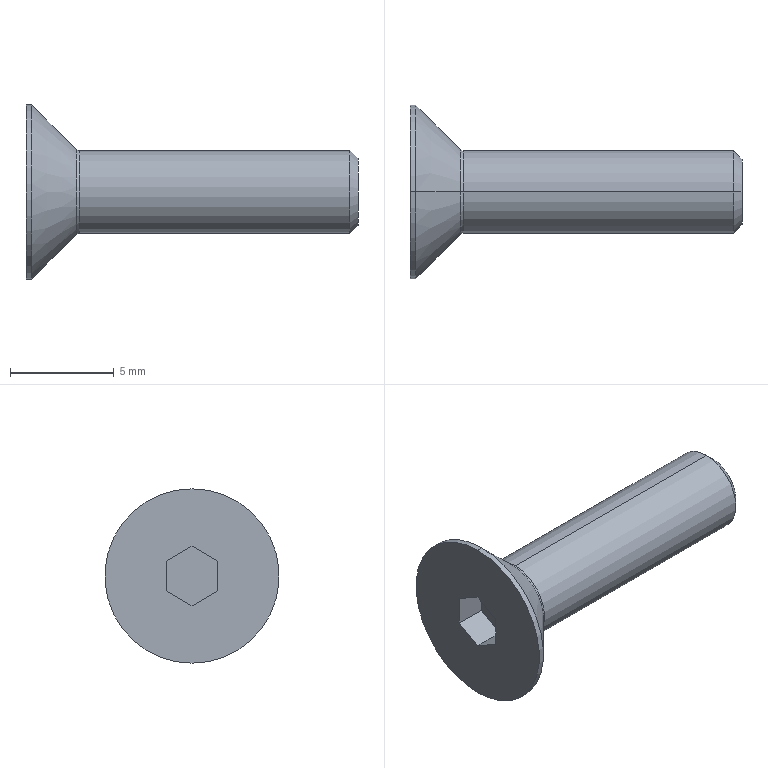Part | STEP file | 1 solid | 19 faces | box 16 x 8.4 x 8.4 mm | volume 245.575 mm3 | plane 9 | cylinder 4 | cone 4 | spline 2 | commonest cylinder face diameters 4 x2 8.4 x2
STEP:
#1=CARTESIAN_POINT('',(0.,0.,0.));
#2=DIRECTION('',(0.,0.,1.));
#3=DIRECTION('',(1.,0.,0.));
#4=AXIS2_PLACEMENT_3D('',#1,#2,#3);
#5=CARTESIAN_POINT('',(-0.98,-1.25,-0.7217));
#6=VERTEX_POINT('',#5);
#7=CARTESIAN_POINT('',(-0.98,-1.25,0.7217));
#8=VERTEX_POINT('',#7);
#9=CARTESIAN_POINT('',(-0.98,-1.25,-0.7217));
#10=DIRECTION('',(0.,0.,1.));
#11=VECTOR('',#10,1.);
#12=LINE('',#9,#11);
#13=CARTESIAN_POINT('',(-0.98,0.,0.));
#14=DIRECTION('',(-1.,0.,0.));
#15=DIRECTION('',(0.,0.,1.));
#16=AXIS2_PLACEMENT_3D('',#13,#14,#15);
#17=PLANE('',#16);
#18=CARTESIAN_POINT('',(-0.7217,-1.25));
#19=DIRECTION('',(1.,0.));
#20=VECTOR('',#19,1.);
#21=LINE('',#18,#20);
#22=(GEOMETRIC_REPRESENTATION_CONTEXT(2)PARAMETRIC_REPRESENTATION_CONTEXT()REPRESENTATION_CONTEXT('',''));
#23=DEFINITIONAL_REPRESENTATION('',(#21),#22);
#24=PCURVE('',#17,#23);
#25=CARTESIAN_POINT('',(-0.98,-1.25,-0.7217));
#26=DIRECTION('',(0.,-1.,0.));
#27=DIRECTION('',(-1.,0.,0.));
#28=AXIS2_PLACEMENT_3D('',#25,#26,#27);
#29=PLANE('',#28);
#30=CARTESIAN_POINT('',(0.,0.));
#31=DIRECTION('',(0.,-1.));
#32=VECTOR('',#31,1.);
#33=LINE('',#30,#32);
#34=(GEOMETRIC_REPRESENTATION_CONTEXT(2)PARAMETRIC_REPRESENTATION_CONTEXT()REPRESENTATION_CONTEXT('',''));
#35=DEFINITIONAL_REPRESENTATION('',(#33),#34);
#36=PCURVE('',#29,#35);
#37=SURFACE_CURVE('',#12,(#24,#36),.PCURVE_S1.);
#38=EDGE_CURVE('',#6,#8,#37,.T.);
#39=ORIENTED_EDGE('',*,*,#38,.T.);
#40=CARTESIAN_POINT('',(-0.98,0.,1.443));
#41=VERTEX_POINT('',#40);
#42=CARTESIAN_POINT('',(-0.98,-1.25,0.7217));
#43=DIRECTION('',(0.,0.866,0.5));
#44=VECTOR('',#43,1.);
#45=LINE('',#42,#44);
#46=CARTESIAN_POINT('',(0.7217,-1.25));
#47=DIRECTION('',(0.5,0.866));
#48=VECTOR('',#47,1.);
#49=LINE('',#46,#48);
#50=(GEOMETRIC_REPRESENTATION_CONTEXT(2)PARAMETRIC_REPRESENTATION_CONTEXT()REPRESENTATION_CONTEXT('',''));
#51=DEFINITIONAL_REPRESENTATION('',(#49),#50);
#52=PCURVE('',#17,#51);
#53=CARTESIAN_POINT('',(-0.98,-1.25,0.7217));
#54=DIRECTION('',(0.,-0.5,0.866));
#55=DIRECTION('',(-1.,0.,0.));
#56=AXIS2_PLACEMENT_3D('',#53,#54,#55);
#57=PLANE('',#56);
#58=CARTESIAN_POINT('',(0.,0.));
#59=DIRECTION('',(0.,-1.));
#60=VECTOR('',#59,1.);
#61=LINE('',#58,#60);
#62=(GEOMETRIC_REPRESENTATION_CONTEXT(2)PARAMETRIC_REPRESENTATION_CONTEXT()REPRESENTATION_CONTEXT('',''));
#63=DEFINITIONAL_REPRESENTATION('',(#61),#62);
#64=PCURVE('',#57,#63);
#65=SURFACE_CURVE('',#45,(#52,#64),.PCURVE_S1.);
#66=EDGE_CURVE('',#8,#41,#65,.T.);
#67=ORIENTED_EDGE('',*,*,#66,.T.);
#68=CARTESIAN_POINT('',(-0.98,1.25,0.7217));
#69=VERTEX_POINT('',#68);
#70=CARTESIAN_POINT('',(-0.98,0.,1.443));
#71=DIRECTION('',(0.,0.866,-0.5));
#72=VECTOR('',#71,1.);
#73=LINE('',#70,#72);
#74=CARTESIAN_POINT('',(1.443,0.));
#75=DIRECTION('',(-0.5,0.866));
#76=VECTOR('',#75,1.);
#77=LINE('',#74,#76);
#78=(GEOMETRIC_REPRESENTATION_CONTEXT(2)PARAMETRIC_REPRESENTATION_CONTEXT()REPRESENTATION_CONTEXT('',''));
#79=DEFINITIONAL_REPRESENTATION('',(#77),#78);
#80=PCURVE('',#17,#79);
#81=CARTESIAN_POINT('',(-0.98,0.,1.443));
#82=DIRECTION('',(0.,0.5,0.866));
#83=DIRECTION('',(1.,0.,0.));
#84=AXIS2_PLACEMENT_3D('',#81,#82,#83);
#85=PLANE('',#84);
#86=CARTESIAN_POINT('',(0.,0.));
#87=DIRECTION('',(0.,1.));
#88=VECTOR('',#87,1.);
#89=LINE('',#86,#88);
#90=(GEOMETRIC_REPRESENTATION_CONTEXT(2)PARAMETRIC_REPRESENTATION_CONTEXT()REPRESENTATION_CONTEXT('',''));
#91=DEFINITIONAL_REPRESENTATION('',(#89),#90);
#92=PCURVE('',#85,#91);
#93=SURFACE_CURVE('',#73,(#80,#92),.PCURVE_S1.);
#94=EDGE_CURVE('',#41,#69,#93,.T.);
#95=ORIENTED_EDGE('',*,*,#94,.T.);
#96=CARTESIAN_POINT('',(-0.98,1.25,-0.7217));
#97=VERTEX_POINT('',#96);
#98=CARTESIAN_POINT('',(-0.98,1.25,0.7217));
#99=DIRECTION('',(0.,0.,-1.));
#100=VECTOR('',#99,1.);
#101=LINE('',#98,#100);
#102=CARTESIAN_POINT('',(0.7217,1.25));
#103=DIRECTION('',(-1.,0.));
#104=VECTOR('',#103,1.);
#105=LINE('',#102,#104);
#106=(GEOMETRIC_REPRESENTATION_CONTEXT(2)PARAMETRIC_REPRESENTATION_CONTEXT()REPRESENTATION_CONTEXT('',''));
#107=DEFINITIONAL_REPRESENTATION('',(#105),#106);
#108=PCURVE('',#17,#107);
#109=CARTESIAN_POINT('',(-0.98,1.25,0.7217));
#110=DIRECTION('',(0.,1.,0.));
#111=DIRECTION('',(1.,0.,0.));
#112=AXIS2_PLACEMENT_3D('',#109,#110,#111);
#113=PLANE('',#112);
#114=CARTESIAN_POINT('',(0.,0.));
#115=DIRECTION('',(0.,1.));
#116=VECTOR('',#115,1.);
#117=LINE('',#114,#116);
#118=(GEOMETRIC_REPRESENTATION_CONTEXT(2)PARAMETRIC_REPRESENTATION_CONTEXT()REPRESENTATION_CONTEXT('',''));
#119=DEFINITIONAL_REPRESENTATION('',(#117),#118);
#120=PCURVE('',#113,#119);
#121=SURFACE_CURVE('',#101,(#108,#120),.PCURVE_S1.);
#122=EDGE_CURVE('',#69,#97,#121,.T.);
#123=ORIENTED_EDGE('',*,*,#122,.T.);
#124=CARTESIAN_POINT('',(-0.98,0.,-1.443));
#125=VERTEX_POINT('',#124);
#126=CARTESIAN_POINT('',(-0.98,1.25,-0.7217));
#127=DIRECTION('',(0.,-0.866,-0.5));
#128=VECTOR('',#127,1.);
#129=LINE('',#126,#128);
#130=CARTESIAN_POINT('',(-0.7217,1.25));
#131=DIRECTION('',(-0.5,-0.866));
#132=VECTOR('',#131,1.);
#133=LINE('',#130,#132);
#134=(GEOMETRIC_REPRESENTATION_CONTEXT(2)PARAMETRIC_REPRESENTATION_CONTEXT()REPRESENTATION_CONTEXT('',''));
#135=DEFINITIONAL_REPRESENTATION('',(#133),#134);
#136=PCURVE('',#17,#135);
#137=CARTESIAN_POINT('',(-0.98,1.25,-0.7217));
#138=DIRECTION('',(0.,0.5,-0.866));
#139=DIRECTION('',(-1.,0.,0.));
#140=AXIS2_PLACEMENT_3D('',#137,#138,#139);
#141=PLANE('',#140);
#142=CARTESIAN_POINT('',(0.,0.));
#143=DIRECTION('',(0.,-1.));
#144=VECTOR('',#143,1.);
#145=LINE('',#142,#144);
#146=(GEOMETRIC_REPRESENTATION_CONTEXT(2)PARAMETRIC_REPRESENTATION_CONTEXT()REPRESENTATION_CONTEXT('',''));
#147=DEFINITIONAL_REPRESENTATION('',(#145),#146);
#148=PCURVE('',#141,#147);
#149=SURFACE_CURVE('',#129,(#136,#148),.PCURVE_S1.);
#150=EDGE_CURVE('',#97,#125,#149,.T.);
#151=ORIENTED_EDGE('',*,*,#150,.T.);
#152=CARTESIAN_POINT('',(-0.98,0.,-1.443));
#153=DIRECTION('',(0.,-0.866,0.5));
#154=VECTOR('',#153,1.);
#155=LINE('',#152,#154);
#156=CARTESIAN_POINT('',(-1.443,0.));
#157=DIRECTION('',(0.5,-0.866));
#158=VECTOR('',#157,1.);
#159=LINE('',#156,#158);
#160=(GEOMETRIC_REPRESENTATION_CONTEXT(2)PARAMETRIC_REPRESENTATION_CONTEXT()REPRESENTATION_CONTEXT('',''));
#161=DEFINITIONAL_REPRESENTATION('',(#159),#160);
#162=PCURVE('',#17,#161);
#163=CARTESIAN_POINT('',(-0.98,0.,-1.443));
#164=DIRECTION('',(0.,-0.5,-0.866));
#165=DIRECTION('',(0.,-0.866,0.5));
#166=AXIS2_PLACEMENT_3D('',#163,#164,#165);
#167=PLANE('',#166);
#168=CARTESIAN_POINT('',(0.,0.));
#169=DIRECTION('',(1.,0.));
#170=VECTOR('',#169,1.);
#171=LINE('',#168,#170);
#172=(GEOMETRIC_REPRESENTATION_CONTEXT(2)PARAMETRIC_REPRESENTATION_CONTEXT()REPRESENTATION_CONTEXT('',''));
#173=DEFINITIONAL_REPRESENTATION('',(#171),#172);
#174=PCURVE('',#167,#173);
#175=SURFACE_CURVE('',#155,(#162,#174),.PCURVE_S1.);
#176=EDGE_CURVE('',#125,#6,#175,.T.);
#177=ORIENTED_EDGE('',*,*,#176,.T.);
#178=EDGE_LOOP('',(#39,#67,#95,#123,#151,#177));
#179=FACE_BOUND('',#178,.T.);
#180=ADVANCED_FACE('',(#179),#17,.T.);
#181=CARTESIAN_POINT('',(-2.48,0.,-1.443));
#182=VERTEX_POINT('',#181);
#183=CARTESIAN_POINT('',(-0.98,0.,-1.443));
#184=DIRECTION('',(1.,0.,0.));
#185=VECTOR('',#184,1.);
#186=LINE('',#183,#185);
#187=CARTESIAN_POINT('',(0.,-1.443));
#188=DIRECTION('',(-1.,0.));
#189=VECTOR('',#188,1.);
#190=LINE('',#187,#189);
#191=(GEOMETRIC_REPRESENTATION_CONTEXT(2)PARAMETRIC_REPRESENTATION_CONTEXT()REPRESENTATION_CONTEXT('',''));
#192=DEFINITIONAL_REPRESENTATION('',(#190),#191);
#193=PCURVE('',#141,#192);
#194=CARTESIAN_POINT('',(0.,0.));
#195=DIRECTION('',(0.,-1.));
#196=VECTOR('',#195,1.);
#197=LINE('',#194,#196);
#198=(GEOMETRIC_REPRESENTATION_CONTEXT(2)PARAMETRIC_REPRESENTATION_CONTEXT()REPRESENTATION_CONTEXT('',''));
#199=DEFINITIONAL_REPRESENTATION('',(#197),#198);
#200=PCURVE('',#167,#199);
#201=SURFACE_CURVE('',#186,(#193,#200),.PCURVE_S1.);
#202=EDGE_CURVE('',#182,#125,#201,.T.);
#203=ORIENTED_EDGE('',*,*,#202,.T.);
#204=ORIENTED_EDGE('',*,*,#150,.F.);
#205=CARTESIAN_POINT('',(-2.48,1.25,-0.7217));
#206=VERTEX_POINT('',#205);
#207=CARTESIAN_POINT('',(-0.98,1.25,-0.7217));
#208=DIRECTION('',(-1.,0.,0.));
#209=VECTOR('',#208,1.);
#210=LINE('',#207,#209);
#211=CARTESIAN_POINT('',(0.,0.));
#212=DIRECTION('',(1.,0.));
#213=VECTOR('',#212,1.);
#214=LINE('',#211,#213);
#215=(GEOMETRIC_REPRESENTATION_CONTEXT(2)PARAMETRIC_REPRESENTATION_CONTEXT()REPRESENTATION_CONTEXT('',''));
#216=DEFINITIONAL_REPRESENTATION('',(#214),#215);
#217=PCURVE('',#141,#216);
#218=CARTESIAN_POINT('',(0.,1.443));
#219=DIRECTION('',(-1.,0.));
#220=VECTOR('',#219,1.);
#221=LINE('',#218,#220);
#222=(GEOMETRIC_REPRESENTATION_CONTEXT(2)PARAMETRIC_REPRESENTATION_CONTEXT()REPRESENTATION_CONTEXT('',''));
#223=DEFINITIONAL_REPRESENTATION('',(#221),#222);
#224=PCURVE('',#113,#223);
#225=SURFACE_CURVE('',#210,(#217,#224),.PCURVE_S1.);
#226=EDGE_CURVE('',#97,#206,#225,.T.);
#227=ORIENTED_EDGE('',*,*,#226,.T.);
#228=CARTESIAN_POINT('',(-2.48,1.25,-0.7217));
#229=DIRECTION('',(0.,-0.866,-0.5));
#230=VECTOR('',#229,1.);
#231=LINE('',#228,#230);
#232=CARTESIAN_POINT('',(1.5,0.));
#233=DIRECTION('',(0.,-1.));
#234=VECTOR('',#233,1.);
#235=LINE('',#232,#234);
#236=(GEOMETRIC_REPRESENTATION_CONTEXT(2)PARAMETRIC_REPRESENTATION_CONTEXT()REPRESENTATION_CONTEXT('',''));
#237=DEFINITIONAL_REPRESENTATION('',(#235),#236);
#238=PCURVE('',#141,#237);
#239=CARTESIAN_POINT('',(-2.48,4.2,0.));
#240=DIRECTION('',(1.,0.,0.));
#241=DIRECTION('',(0.,1.,0.));
#242=AXIS2_PLACEMENT_3D('',#239,#240,#241);
#243=PLANE('',#242);
#244=CARTESIAN_POINT('',(-2.95,-0.7217));
#245=DIRECTION('',(-0.866,-0.5));
#246=VECTOR('',#245,1.);
#247=LINE('',#244,#246);
#248=(GEOMETRIC_REPRESENTATION_CONTEXT(2)PARAMETRIC_REPRESENTATION_CONTEXT()REPRESENTATION_CONTEXT('',''));
#249=DEFINITIONAL_REPRESENTATION('',(#247),#248);
#250=PCURVE('',#243,#249);
#251=SURFACE_CURVE('',#231,(#238,#250),.PCURVE_S1.);
#252=EDGE_CURVE('',#206,#182,#251,.T.);
#253=ORIENTED_EDGE('',*,*,#252,.T.);
#254=EDGE_LOOP('',(#203,#204,#227,#253));
#255=FACE_BOUND('',#254,.T.);
#256=ADVANCED_FACE('',(#255),#141,.F.);
#257=CARTESIAN_POINT('',(-2.48,-1.25,-0.7217));
#258=VERTEX_POINT('',#257);
#259=CARTESIAN_POINT('',(-0.98,-1.25,-0.7217));
#260=DIRECTION('',(1.,0.,0.));
#261=VECTOR('',#260,1.);
#262=LINE('',#259,#261);
#263=CARTESIAN_POINT('',(1.443,0.));
#264=DIRECTION('',(0.,-1.));
#265=VECTOR('',#264,1.);
#266=LINE('',#263,#265);
#267=(GEOMETRIC_REPRESENTATION_CONTEXT(2)PARAMETRIC_REPRESENTATION_CONTEXT()REPRESENTATION_CONTEXT('',''));
#268=DEFINITIONAL_REPRESENTATION('',(#266),#267);
#269=PCURVE('',#167,#268);
#270=CARTESIAN_POINT('',(0.,0.));
#271=DIRECTION('',(-1.,0.));
#272=VECTOR('',#271,1.);
#273=LINE('',#270,#272);
#274=(GEOMETRIC_REPRESENTATION_CONTEXT(2)PARAMETRIC_REPRESENTATION_CONTEXT()REPRESENTATION_CONTEXT('',''));
#275=DEFINITIONAL_REPRESENTATION('',(#273),#274);
#276=PCURVE('',#29,#275);
#277=SURFACE_CURVE('',#262,(#269,#276),.PCURVE_S1.);
#278=EDGE_CURVE('',#258,#6,#277,.T.);
#279=ORIENTED_EDGE('',*,*,#278,.T.);
#280=ORIENTED_EDGE('',*,*,#176,.F.);
#281=ORIENTED_EDGE('',*,*,#202,.F.);
#282=CARTESIAN_POINT('',(-2.48,0.,-1.443));
#283=DIRECTION('',(0.,-0.866,0.5));
#284=VECTOR('',#283,1.);
#285=LINE('',#282,#284);
#286=CARTESIAN_POINT('',(0.,1.5));
#287=DIRECTION('',(1.,0.));
#288=VECTOR('',#287,1.);
#289=LINE('',#286,#288);
#290=(GEOMETRIC_REPRESENTATION_CONTEXT(2)PARAMETRIC_REPRESENTATION_CONTEXT()REPRESENTATION_CONTEXT('',''));
#291=DEFINITIONAL_REPRESENTATION('',(#289),#290);
#292=PCURVE('',#167,#291);
#293=CARTESIAN_POINT('',(-4.2,-1.443));
#294=DIRECTION('',(-0.866,0.5));
#295=VECTOR('',#294,1.);
#296=LINE('',#293,#295);
#297=(GEOMETRIC_REPRESENTATION_CONTEXT(2)PARAMETRIC_REPRESENTATION_CONTEXT()REPRESENTATION_CONTEXT('',''));
#298=DEFINITIONAL_REPRESENTATION('',(#296),#297);
#299=PCURVE('',#243,#298);
#300=SURFACE_CURVE('',#285,(#292,#299),.PCURVE_S1.);
#301=EDGE_CURVE('',#182,#258,#300,.T.);
#302=ORIENTED_EDGE('',*,*,#301,.T.);
#303=EDGE_LOOP('',(#279,#280,#281,#302));
#304=FACE_BOUND('',#303,.T.);
#305=ADVANCED_FACE('',(#304),#167,.F.);
#306=CARTESIAN_POINT('',(-2.48,-1.25,0.7217));
#307=VERTEX_POINT('',#306);
#308=CARTESIAN_POINT('',(-0.98,-1.25,0.7217));
#309=DIRECTION('',(1.,0.,0.));
#310=VECTOR('',#309,1.);
#311=LINE('',#308,#310);
#312=CARTESIAN_POINT('',(0.,-1.443));
#313=DIRECTION('',(-1.,0.));
#314=VECTOR('',#313,1.);
#315=LINE('',#312,#314);
#316=(GEOMETRIC_REPRESENTATION_CONTEXT(2)PARAMETRIC_REPRESENTATION_CONTEXT()REPRESENTATION_CONTEXT('',''));
#317=DEFINITIONAL_REPRESENTATION('',(#315),#316);
#318=PCURVE('',#29,#317);
#319=CARTESIAN_POINT('',(0.,0.));
#320=DIRECTION('',(-1.,0.));
#321=VECTOR('',#320,1.);
#322=LINE('',#319,#321);
#323=(GEOMETRIC_REPRESENTATION_CONTEXT(2)PARAMETRIC_REPRESENTATION_CONTEXT()REPRESENTATION_CONTEXT('',''));
#324=DEFINITIONAL_REPRESENTATION('',(#322),#323);
#325=PCURVE('',#57,#324);
#326=SURFACE_CURVE('',#311,(#318,#325),.PCURVE_S1.);
#327=EDGE_CURVE('',#307,#8,#326,.T.);
#328=ORIENTED_EDGE('',*,*,#327,.T.);
#329=ORIENTED_EDGE('',*,*,#38,.F.);
#330=ORIENTED_EDGE('',*,*,#278,.F.);
#331=CARTESIAN_POINT('',(-2.48,-1.25,0.));
#332=DIRECTION('',(0.,0.,1.));
#333=VECTOR('',#332,1.);
#334=LINE('',#331,#333);
#335=CARTESIAN_POINT('',(1.5,-0.7217));
#336=DIRECTION('',(0.,-1.));
#337=VECTOR('',#336,1.);
#338=LINE('',#335,#337);
#339=(GEOMETRIC_REPRESENTATION_CONTEXT(2)PARAMETRIC_REPRESENTATION_CONTEXT()REPRESENTATION_CONTEXT('',''));
#340=DEFINITIONAL_REPRESENTATION('',(#338),#339);
#341=PCURVE('',#29,#340);
#342=CARTESIAN_POINT('',(-5.45,0.));
#343=DIRECTION('',(0.,1.));
#344=VECTOR('',#343,1.);
#345=LINE('',#342,#344);
#346=(GEOMETRIC_REPRESENTATION_CONTEXT(2)PARAMETRIC_REPRESENTATION_CONTEXT()REPRESENTATION_CONTEXT('',''));
#347=DEFINITIONAL_REPRESENTATION('',(#345),#346);
#348=PCURVE('',#243,#347);
#349=SURFACE_CURVE('',#334,(#341,#348),.PCURVE_S1.);
#350=EDGE_CURVE('',#258,#307,#349,.T.);
#351=ORIENTED_EDGE('',*,*,#350,.T.);
#352=EDGE_LOOP('',(#328,#329,#330,#351));
#353=FACE_BOUND('',#352,.T.);
#354=ADVANCED_FACE('',(#353),#29,.F.);
#355=CARTESIAN_POINT('',(-2.48,0.,1.443));
#356=VERTEX_POINT('',#355);
#357=CARTESIAN_POINT('',(-0.98,0.,1.443));
#358=DIRECTION('',(1.,0.,0.));
#359=VECTOR('',#358,1.);
#360=LINE('',#357,#359);
#361=CARTESIAN_POINT('',(0.,-1.443));
#362=DIRECTION('',(-1.,0.));
#363=VECTOR('',#362,1.);
#364=LINE('',#361,#363);
#365=(GEOMETRIC_REPRESENTATION_CONTEXT(2)PARAMETRIC_REPRESENTATION_CONTEXT()REPRESENTATION_CONTEXT('',''));
#366=DEFINITIONAL_REPRESENTATION('',(#364),#365);
#367=PCURVE('',#57,#366);
#368=CARTESIAN_POINT('',(0.,0.));
#369=DIRECTION('',(1.,0.));
#370=VECTOR('',#369,1.);
#371=LINE('',#368,#370);
#372=(GEOMETRIC_REPRESENTATION_CONTEXT(2)PARAMETRIC_REPRESENTATION_CONTEXT()REPRESENTATION_CONTEXT('',''));
#373=DEFINITIONAL_REPRESENTATION('',(#371),#372);
#374=PCURVE('',#85,#373);
#375=SURFACE_CURVE('',#360,(#367,#374),.PCURVE_S1.);
#376=EDGE_CURVE('',#356,#41,#375,.T.);
#377=ORIENTED_EDGE('',*,*,#376,.T.);
#378=ORIENTED_EDGE('',*,*,#66,.F.);
#379=ORIENTED_EDGE('',*,*,#327,.F.);
#380=CARTESIAN_POINT('',(-2.48,-1.25,0.7217));
#381=DIRECTION('',(0.,0.866,0.5));
#382=VECTOR('',#381,1.);
#383=LINE('',#380,#382);
#384=CARTESIAN_POINT('',(1.5,0.));
#385=DIRECTION('',(0.,-1.));
#386=VECTOR('',#385,1.);
#387=LINE('',#384,#386);
#388=(GEOMETRIC_REPRESENTATION_CONTEXT(2)PARAMETRIC_REPRESENTATION_CONTEXT()REPRESENTATION_CONTEXT('',''));
#389=DEFINITIONAL_REPRESENTATION('',(#387),#388);
#390=PCURVE('',#57,#389);
#391=CARTESIAN_POINT('',(-5.45,0.7217));
#392=DIRECTION('',(0.866,0.5));
#393=VECTOR('',#392,1.);
#394=LINE('',#391,#393);
#395=(GEOMETRIC_REPRESENTATION_CONTEXT(2)PARAMETRIC_REPRESENTATION_CONTEXT()REPRESENTATION_CONTEXT('',''));
#396=DEFINITIONAL_REPRESENTATION('',(#394),#395);
#397=PCURVE('',#243,#396);
#398=SURFACE_CURVE('',#383,(#390,#397),.PCURVE_S1.);
#399=EDGE_CURVE('',#307,#356,#398,.T.);
#400=ORIENTED_EDGE('',*,*,#399,.T.);
#401=EDGE_LOOP('',(#377,#378,#379,#400));
#402=FACE_BOUND('',#401,.T.);
#403=ADVANCED_FACE('',(#402),#57,.F.);
#404=CARTESIAN_POINT('',(-2.48,1.25,0.7217));
#405=VERTEX_POINT('',#404);
#406=CARTESIAN_POINT('',(-0.98,1.25,0.7217));
#407=DIRECTION('',(1.,0.,0.));
#408=VECTOR('',#407,1.);
#409=LINE('',#406,#408);
#410=CARTESIAN_POINT('',(0.,1.443));
#411=DIRECTION('',(1.,0.));
#412=VECTOR('',#411,1.);
#413=LINE('',#410,#412);
#414=(GEOMETRIC_REPRESENTATION_CONTEXT(2)PARAMETRIC_REPRESENTATION_CONTEXT()REPRESENTATION_CONTEXT('',''));
#415=DEFINITIONAL_REPRESENTATION('',(#413),#414);
#416=PCURVE('',#85,#415);
#417=CARTESIAN_POINT('',(0.,0.));
#418=DIRECTION('',(1.,0.));
#419=VECTOR('',#418,1.);
#420=LINE('',#417,#419);
#421=(GEOMETRIC_REPRESENTATION_CONTEXT(2)PARAMETRIC_REPRESENTATION_CONTEXT()REPRESENTATION_CONTEXT('',''));
#422=DEFINITIONAL_REPRESENTATION('',(#420),#421);
#423=PCURVE('',#113,#422);
#424=SURFACE_CURVE('',#409,(#416,#423),.PCURVE_S1.);
#425=EDGE_CURVE('',#405,#69,#424,.T.);
#426=ORIENTED_EDGE('',*,*,#425,.T.);
#427=ORIENTED_EDGE('',*,*,#94,.F.);
#428=ORIENTED_EDGE('',*,*,#376,.F.);
#429=CARTESIAN_POINT('',(-2.48,0.,1.443));
#430=DIRECTION('',(0.,0.866,-0.5));
#431=VECTOR('',#430,1.);
#432=LINE('',#429,#431);
#433=CARTESIAN_POINT('',(-1.5,0.));
#434=DIRECTION('',(0.,1.));
#435=VECTOR('',#434,1.);
#436=LINE('',#433,#435);
#437=(GEOMETRIC_REPRESENTATION_CONTEXT(2)PARAMETRIC_REPRESENTATION_CONTEXT()REPRESENTATION_CONTEXT('',''));
#438=DEFINITIONAL_REPRESENTATION('',(#436),#437);
#439=PCURVE('',#85,#438);
#440=CARTESIAN_POINT('',(-4.2,1.443));
#441=DIRECTION('',(0.866,-0.5));
#442=VECTOR('',#441,1.);
#443=LINE('',#440,#442);
#444=(GEOMETRIC_REPRESENTATION_CONTEXT(2)PARAMETRIC_REPRESENTATION_CONTEXT()REPRESENTATION_CONTEXT('',''));
#445=DEFINITIONAL_REPRESENTATION('',(#443),#444);
#446=PCURVE('',#243,#445);
#447=SURFACE_CURVE('',#432,(#439,#446),.PCURVE_S1.);
#448=EDGE_CURVE('',#356,#405,#447,.T.);
#449=ORIENTED_EDGE('',*,*,#448,.T.);
#450=EDGE_LOOP('',(#426,#427,#428,#449));
#451=FACE_BOUND('',#450,.T.);
#452=ADVANCED_FACE('',(#451),#85,.F.);
#453=ORIENTED_EDGE('',*,*,#226,.F.);
#454=ORIENTED_EDGE('',*,*,#122,.F.);
#455=ORIENTED_EDGE('',*,*,#425,.F.);
#456=CARTESIAN_POINT('',(-2.48,1.25,0.));
#457=DIRECTION('',(0.,0.,-1.));
#458=VECTOR('',#457,1.);
#459=LINE('',#456,#458);
#460=CARTESIAN_POINT('',(-1.5,0.7217));
#461=DIRECTION('',(0.,1.));
#462=VECTOR('',#461,1.);
#463=LINE('',#460,#462);
#464=(GEOMETRIC_REPRESENTATION_CONTEXT(2)PARAMETRIC_REPRESENTATION_CONTEXT()REPRESENTATION_CONTEXT('',''));
#465=DEFINITIONAL_REPRESENTATION('',(#463),#464);
#466=PCURVE('',#113,#465);
#467=CARTESIAN_POINT('',(-2.95,0.));
#468=DIRECTION('',(0.,-1.));
#469=VECTOR('',#468,1.);
#470=LINE('',#467,#469);
#471=(GEOMETRIC_REPRESENTATION_CONTEXT(2)PARAMETRIC_REPRESENTATION_CONTEXT()REPRESENTATION_CONTEXT('',''));
#472=DEFINITIONAL_REPRESENTATION('',(#470),#471);
#473=PCURVE('',#243,#472);
#474=SURFACE_CURVE('',#459,(#466,#473),.PCURVE_S1.);
#475=EDGE_CURVE('',#405,#206,#474,.T.);
#476=ORIENTED_EDGE('',*,*,#475,.T.);
#477=EDGE_LOOP('',(#453,#454,#455,#476));
#478=FACE_BOUND('',#477,.T.);
#479=ADVANCED_FACE('',(#478),#113,.F.);
#480=ORIENTED_EDGE('',*,*,#448,.F.);
#481=ORIENTED_EDGE('',*,*,#399,.F.);
#482=ORIENTED_EDGE('',*,*,#350,.F.);
#483=ORIENTED_EDGE('',*,*,#301,.F.);
#484=ORIENTED_EDGE('',*,*,#252,.F.);
#485=ORIENTED_EDGE('',*,*,#475,.F.);
#486=EDGE_LOOP('',(#480,#481,#482,#483,#484,#485));
#487=FACE_BOUND('',#486,.T.);
#488=CARTESIAN_POINT('',(-2.48,0.,4.2));
#489=VERTEX_POINT('',#488);
#490=CARTESIAN_POINT('',(-2.48,0.,-4.2));
#491=VERTEX_POINT('',#490);
#492=CARTESIAN_POINT('',(-2.48,0.,0.));
#493=DIRECTION('',(1.,0.,0.));
#494=DIRECTION('',(0.,0.,1.));
#495=AXIS2_PLACEMENT_3D('',#492,#493,#494);
#496=CIRCLE('',#495,4.2);
#497=CARTESIAN_POINT('',(-4.2,0.));
#498=DIRECTION('',(0.,1.));
#499=AXIS2_PLACEMENT_2D('',#497,#498);
#500=CIRCLE('',#499,4.2);
#501=(GEOMETRIC_REPRESENTATION_CONTEXT(2)PARAMETRIC_REPRESENTATION_CONTEXT()REPRESENTATION_CONTEXT('',''));
#502=DEFINITIONAL_REPRESENTATION('',(#500),#501);
#503=PCURVE('',#243,#502);
#504=CARTESIAN_POINT('',(-21.552,0.,0.));
#505=DIRECTION('',(-1.,0.,0.));
#506=DIRECTION('',(0.,0.,1.));
#507=AXIS2_PLACEMENT_3D('',#504,#505,#506);
#508=CYLINDRICAL_SURFACE('',#507,4.2);
#509=CARTESIAN_POINT('',(6.283,-19.072));
#510=DIRECTION('',(-1.,0.));
#511=VECTOR('',#510,1.);
#512=LINE('',#509,#511);
#513=(GEOMETRIC_REPRESENTATION_CONTEXT(2)PARAMETRIC_REPRESENTATION_CONTEXT()REPRESENTATION_CONTEXT('',''));
#514=DEFINITIONAL_REPRESENTATION('',(#512),#513);
#515=PCURVE('',#508,#514);
#516=SURFACE_CURVE('',#496,(#503,#515),.PCURVE_S1.);
#517=EDGE_CURVE('',#489,#491,#516,.T.);
#518=ORIENTED_EDGE('',*,*,#517,.F.);
#519=CARTESIAN_POINT('',(-2.48,0.,0.));
#520=DIRECTION('',(1.,0.,0.));
#521=DIRECTION('',(0.,0.,1.));
#522=AXIS2_PLACEMENT_3D('',#519,#520,#521);
#523=CIRCLE('',#522,4.2);
#524=CARTESIAN_POINT('',(-4.2,0.));
#525=DIRECTION('',(0.,1.));
#526=AXIS2_PLACEMENT_2D('',#524,#525);
#527=CIRCLE('',#526,4.2);
#528=(GEOMETRIC_REPRESENTATION_CONTEXT(2)PARAMETRIC_REPRESENTATION_CONTEXT()REPRESENTATION_CONTEXT('',''));
#529=DEFINITIONAL_REPRESENTATION('',(#527),#528);
#530=PCURVE('',#243,#529);
#531=CARTESIAN_POINT('',(-21.552,0.,0.));
#532=DIRECTION('',(-1.,0.,0.));
#533=DIRECTION('',(0.,0.,1.));
#534=AXIS2_PLACEMENT_3D('',#531,#532,#533);
#535=CYLINDRICAL_SURFACE('',#534,4.2);
#536=CARTESIAN_POINT('',(6.283,-19.072));
#537=DIRECTION('',(-1.,0.));
#538=VECTOR('',#537,1.);
#539=LINE('',#536,#538);
#540=(GEOMETRIC_REPRESENTATION_CONTEXT(2)PARAMETRIC_REPRESENTATION_CONTEXT()REPRESENTATION_CONTEXT('',''));
#541=DEFINITIONAL_REPRESENTATION('',(#539),#540);
#542=PCURVE('',#535,#541);
#543=SURFACE_CURVE('',#523,(#530,#542),.PCURVE_S1.);
#544=EDGE_CURVE('',#491,#489,#543,.T.);
#545=ORIENTED_EDGE('',*,*,#544,.F.);
#546=EDGE_LOOP('',(#518,#545));
#547=FACE_BOUND('',#546,.T.);
#548=ADVANCED_FACE('',(#487,#547),#243,.F.);
#549=CARTESIAN_POINT('',(-2.2,0.,-4.2));
#550=VERTEX_POINT('',#549);
#551=CARTESIAN_POINT('',(-21.552,0.,-4.2));
#552=DIRECTION('',(-1.,0.,0.));
#553=VECTOR('',#552,1.);
#554=LINE('',#551,#553);
#555=CARTESIAN_POINT('',(3.142,0.));
#556=DIRECTION('',(0.,1.));
#557=VECTOR('',#556,1.);
#558=LINE('',#555,#557);
#559=(GEOMETRIC_REPRESENTATION_CONTEXT(2)PARAMETRIC_REPRESENTATION_CONTEXT()REPRESENTATION_CONTEXT('',''));
#560=DEFINITIONAL_REPRESENTATION('',(#558),#559);
#561=PCURVE('',#508,#560);
#562=CARTESIAN_POINT('',(3.142,0.));
#563=DIRECTION('',(0.,1.));
#564=VECTOR('',#563,1.);
#565=LINE('',#562,#564);
#566=(GEOMETRIC_REPRESENTATION_CONTEXT(2)PARAMETRIC_REPRESENTATION_CONTEXT()REPRESENTATION_CONTEXT('',''));
#567=DEFINITIONAL_REPRESENTATION('',(#565),#566);
#568=PCURVE('',#535,#567);
#569=SURFACE_CURVE('',#554,(#561,#568),.PCURVE_S1.);
#570=EDGE_CURVE('',#550,#491,#569,.T.);
#571=ORIENTED_EDGE('',*,*,#570,.F.);
#572=CARTESIAN_POINT('',(-2.2,0.,4.2));
#573=VERTEX_POINT('',#572);
#574=CARTESIAN_POINT('',(-2.2,0.,0.));
#575=DIRECTION('',(1.,0.,0.));
#576=DIRECTION('',(0.,0.,1.));
#577=AXIS2_PLACEMENT_3D('',#574,#575,#576);
#578=CIRCLE('',#577,4.2);
#579=CARTESIAN_POINT('',(6.283,-19.352));
#580=DIRECTION('',(-1.,0.));
#581=VECTOR('',#580,1.);
#582=LINE('',#579,#581);
#583=(GEOMETRIC_REPRESENTATION_CONTEXT(2)PARAMETRIC_REPRESENTATION_CONTEXT()REPRESENTATION_CONTEXT('',''));
#584=DEFINITIONAL_REPRESENTATION('',(#582),#583);
#585=PCURVE('',#508,#584);
#586=CARTESIAN_POINT('',(-2.2,0.,0.));
#587=DIRECTION('',(-1.,0.,0.));
#588=DIRECTION('',(0.,0.,1.));
#589=AXIS2_PLACEMENT_3D('',#586,#587,#588);
#590=CONICAL_SURFACE('',#589,4.2,0.7854);
#591=CARTESIAN_POINT('',(6.283,0.));
#592=DIRECTION('',(-1.,0.));
#593=VECTOR('',#592,1.);
#594=LINE('',#591,#593);
#595=(GEOMETRIC_REPRESENTATION_CONTEXT(2)PARAMETRIC_REPRESENTATION_CONTEXT()REPRESENTATION_CONTEXT('',''));
#596=DEFINITIONAL_REPRESENTATION('',(#594),#595);
#597=PCURVE('',#590,#596);
#598=SURFACE_CURVE('',#578,(#585,#597),.PCURVE_S1.);
#599=EDGE_CURVE('',#573,#550,#598,.T.);
#600=ORIENTED_EDGE('',*,*,#599,.F.);
#601=CARTESIAN_POINT('',(-21.552,0.,4.2));
#602=DIRECTION('',(-1.,0.,0.));
#603=VECTOR('',#602,1.);
#604=LINE('',#601,#603);
#605=CARTESIAN_POINT('',(6.283,0.));
#606=DIRECTION('',(0.,1.));
#607=VECTOR('',#606,1.);
#608=LINE('',#605,#607);
#609=(GEOMETRIC_REPRESENTATION_CONTEXT(2)PARAMETRIC_REPRESENTATION_CONTEXT()REPRESENTATION_CONTEXT('',''));
#610=DEFINITIONAL_REPRESENTATION('',(#608),#609);
#611=PCURVE('',#508,#610);
#612=CARTESIAN_POINT('',(0.,0.));
#613=DIRECTION('',(0.,1.));
#614=VECTOR('',#613,1.);
#615=LINE('',#612,#614);
#616=(GEOMETRIC_REPRESENTATION_CONTEXT(2)PARAMETRIC_REPRESENTATION_CONTEXT()REPRESENTATION_CONTEXT('',''));
#617=DEFINITIONAL_REPRESENTATION('',(#615),#616);
#618=PCURVE('',#535,#617);
#619=SURFACE_CURVE('',#604,(#611,#618),.PCURVE_S1.);
#620=EDGE_CURVE('',#573,#489,#619,.T.);
#621=ORIENTED_EDGE('',*,*,#620,.T.);
#622=ORIENTED_EDGE('',*,*,#517,.T.);
#623=EDGE_LOOP('',(#571,#600,#621,#622));
#624=FACE_BOUND('',#623,.T.);
#625=ADVANCED_FACE('',(#624),#508,.T.);
#626=CARTESIAN_POINT('',(13.52,0.,1.6));
#627=VERTEX_POINT('',#626);
#628=CARTESIAN_POINT('',(13.52,0.,-1.6));
#629=VERTEX_POINT('',#628);
#630=CARTESIAN_POINT('',(13.52,0.,0.));
#631=DIRECTION('',(-1.,0.,0.));
#632=DIRECTION('',(0.,0.,1.));
#633=AXIS2_PLACEMENT_3D('',#630,#631,#632);
#634=CIRCLE('',#633,1.6);
#635=CARTESIAN_POINT('',(13.52,2.,0.));
#636=DIRECTION('',(-1.,0.,0.));
#637=DIRECTION('',(0.,0.,1.));
#638=AXIS2_PLACEMENT_3D('',#635,#636,#637);
#639=PLANE('',#638);
#640=CARTESIAN_POINT('',(0.,-2.));
#641=DIRECTION('',(1.,0.));
#642=AXIS2_PLACEMENT_2D('',#640,#641);
#643=CIRCLE('',#642,1.6);
#644=(GEOMETRIC_REPRESENTATION_CONTEXT(2)PARAMETRIC_REPRESENTATION_CONTEXT()REPRESENTATION_CONTEXT('',''));
#645=DEFINITIONAL_REPRESENTATION('',(#643),#644);
#646=PCURVE('',#639,#645);
#647=CARTESIAN_POINT('',(13.12,0.,0.));
#648=DIRECTION('',(-1.,0.,0.));
#649=DIRECTION('',(0.,0.,1.));
#650=AXIS2_PLACEMENT_3D('',#647,#648,#649);
#651=CONICAL_SURFACE('',#650,2.,0.7854);
#652=CARTESIAN_POINT('',(0.,-0.4));
#653=DIRECTION('',(1.,0.));
#654=VECTOR('',#653,1.);
#655=LINE('',#652,#654);
#656=(GEOMETRIC_REPRESENTATION_CONTEXT(2)PARAMETRIC_REPRESENTATION_CONTEXT()REPRESENTATION_CONTEXT('',''));
#657=DEFINITIONAL_REPRESENTATION('',(#655),#656);
#658=PCURVE('',#651,#657);
#659=SURFACE_CURVE('',#634,(#646,#658),.PCURVE_S1.);
#660=EDGE_CURVE('',#627,#629,#659,.T.);
#661=ORIENTED_EDGE('',*,*,#660,.F.);
#662=CARTESIAN_POINT('',(13.52,0.,0.));
#663=DIRECTION('',(-1.,0.,0.));
#664=DIRECTION('',(0.,0.,1.));
#665=AXIS2_PLACEMENT_3D('',#662,#663,#664);
#666=CIRCLE('',#665,1.6);
#667=CARTESIAN_POINT('',(0.,-2.));
#668=DIRECTION('',(1.,0.));
#669=AXIS2_PLACEMENT_2D('',#667,#668);
#670=CIRCLE('',#669,1.6);
#671=(GEOMETRIC_REPRESENTATION_CONTEXT(2)PARAMETRIC_REPRESENTATION_CONTEXT()REPRESENTATION_CONTEXT('',''));
#672=DEFINITIONAL_REPRESENTATION('',(#670),#671);
#673=PCURVE('',#639,#672);
#674=CARTESIAN_POINT('',(13.12,0.,0.));
#675=DIRECTION('',(-1.,0.,0.));
#676=DIRECTION('',(0.,0.,1.));
#677=AXIS2_PLACEMENT_3D('',#674,#675,#676);
#678=CONICAL_SURFACE('',#677,2.,0.7854);
#679=CARTESIAN_POINT('',(0.,-0.4));
#680=DIRECTION('',(1.,0.));
#681=VECTOR('',#680,1.);
#682=LINE('',#679,#681);
#683=(GEOMETRIC_REPRESENTATION_CONTEXT(2)PARAMETRIC_REPRESENTATION_CONTEXT()REPRESENTATION_CONTEXT('',''));
#684=DEFINITIONAL_REPRESENTATION('',(#682),#683);
#685=PCURVE('',#678,#684);
#686=SURFACE_CURVE('',#666,(#673,#685),.PCURVE_S1.);
#687=EDGE_CURVE('',#629,#627,#686,.T.);
#688=ORIENTED_EDGE('',*,*,#687,.F.);
#689=EDGE_LOOP('',(#661,#688));
#690=FACE_BOUND('',#689,.T.);
#691=ADVANCED_FACE('',(#690),#639,.F.);
#692=CARTESIAN_POINT('',(-0.05858,0.,-2.059));
#693=VERTEX_POINT('',#692);
#694=CARTESIAN_POINT('',(-2.2,0.,-4.2));
#695=DIRECTION('',(-0.7071,0.,-0.7071));
#696=VECTOR('',#695,1.);
#697=LINE('',#694,#696);
#698=CARTESIAN_POINT('',(3.142,0.));
#699=DIRECTION('',(0.,1.));
#700=VECTOR('',#699,1.);
#701=LINE('',#698,#700);
#702=(GEOMETRIC_REPRESENTATION_CONTEXT(2)PARAMETRIC_REPRESENTATION_CONTEXT()REPRESENTATION_CONTEXT('',''));
#703=DEFINITIONAL_REPRESENTATION('',(#701),#702);
#704=PCURVE('',#590,#703);
#705=CARTESIAN_POINT('',(-2.2,0.,0.));
#706=DIRECTION('',(-1.,0.,0.));
#707=DIRECTION('',(0.,0.,1.));
#708=AXIS2_PLACEMENT_3D('',#705,#706,#707);
#709=CONICAL_SURFACE('',#708,4.2,0.7854);
#710=CARTESIAN_POINT('',(3.142,0.));
#711=DIRECTION('',(0.,1.));
#712=VECTOR('',#711,1.);
#713=LINE('',#710,#712);
#714=(GEOMETRIC_REPRESENTATION_CONTEXT(2)PARAMETRIC_REPRESENTATION_CONTEXT()REPRESENTATION_CONTEXT('',''));
#715=DEFINITIONAL_REPRESENTATION('',(#713),#714);
#716=PCURVE('',#709,#715);
#717=SURFACE_CURVE('',#697,(#704,#716),.PCURVE_S1.);
#718=EDGE_CURVE('',#693,#550,#717,.T.);
#719=ORIENTED_EDGE('',*,*,#718,.F.);
#720=CARTESIAN_POINT('',(-0.05858,0.,2.059));
#721=VERTEX_POINT('',#720);
#722=CARTESIAN_POINT('',(-0.05858,0.,0.));
#723=DIRECTION('',(-1.,0.,0.));
#724=DIRECTION('',(0.,0.,1.));
#725=AXIS2_PLACEMENT_3D('',#722,#723,#724);
#726=CIRCLE('',#725,2.059);
#727=CARTESIAN_POINT('',(0.,-2.141));
#728=DIRECTION('',(1.,0.));
#729=VECTOR('',#728,1.);
#730=LINE('',#727,#729);
#731=(GEOMETRIC_REPRESENTATION_CONTEXT(2)PARAMETRIC_REPRESENTATION_CONTEXT()REPRESENTATION_CONTEXT('',''));
#732=DEFINITIONAL_REPRESENTATION('',(#730),#731);
#733=PCURVE('',#590,#732);
#734=CARTESIAN_POINT('',(0.08284,0.,-2.));
#735=CARTESIAN_POINT('',(0.08284,-4.,-2.));
#736=CARTESIAN_POINT('',(0.08284,-4.,2.));
#737=CARTESIAN_POINT('',(0.08284,0.,2.));
#738=CARTESIAN_POINT('',(0.02909,0.,-2.));
#739=CARTESIAN_POINT('',(0.02909,-4.,-2.));
#740=CARTESIAN_POINT('',(0.02909,-4.,2.));
#741=CARTESIAN_POINT('',(0.02909,0.,2.));
#742=CARTESIAN_POINT('',(-0.02057,0.,-2.021));
#743=CARTESIAN_POINT('',(-0.02057,-4.041,-2.021));
#744=CARTESIAN_POINT('',(-0.02057,-4.041,2.021));
#745=CARTESIAN_POINT('',(-0.02057,0.,2.021));
#746=CARTESIAN_POINT('',(-0.05858,0.,-2.059));
#747=CARTESIAN_POINT('',(-0.05858,-4.117,-2.059));
#748=CARTESIAN_POINT('',(-0.05858,-4.117,2.059));
#749=CARTESIAN_POINT('',(-0.05858,0.,2.059));
#750=(BOUNDED_SURFACE()B_SPLINE_SURFACE(3,3,((#734,#735,#736,#737),(#738,#739,#740,#741),(#742,#743,#744,#745),(#746,#747,#748,#749)),.UNSPECIFIED.,.F.,.F.,.F.)B_SPLINE_SURFACE_WITH_KNOTS((4,4),(4,4),(0.,1.),(0.,1.),.PIECEWISE_BEZIER_KNOTS.)GEOMETRIC_REPRESENTATION_ITEM()RATIONAL_B_SPLINE_SURFACE(((1.,0.3333,0.3333,1.),(0.9493,0.3164,0.3164,0.9493),(0.9493,0.3164,0.3164,0.9493),(1.,0.3333,0.3333,1.)))REPRESENTATION_ITEM('')SURFACE());
#751=CARTESIAN_POINT('',(1.,0.));
#752=CARTESIAN_POINT('',(1.,0.02375));
#753=CARTESIAN_POINT('',(1.,0.06805));
#754=CARTESIAN_POINT('',(1.,0.1267));
#755=CARTESIAN_POINT('',(1.,0.1794));
#756=CARTESIAN_POINT('',(1.,0.2276));
#757=CARTESIAN_POINT('',(1.,0.2721));
#758=CARTESIAN_POINT('',(1.,0.3139));
#759=CARTESIAN_POINT('',(1.,0.3535));
#760=CARTESIAN_POINT('',(1.,0.3914));
#761=CARTESIAN_POINT('',(1.,0.4282));
#762=CARTESIAN_POINT('',(1.,0.4643));
#763=CARTESIAN_POINT('',(1.,0.5));
#764=CARTESIAN_POINT('',(1.,0.5357));
#765=CARTESIAN_POINT('',(1.,0.5718));
#766=CARTESIAN_POINT('',(1.,0.6086));
#767=CARTESIAN_POINT('',(1.,0.6465));
#768=CARTESIAN_POINT('',(1.,0.6861));
#769=CARTESIAN_POINT('',(1.,0.7279));
#770=CARTESIAN_POINT('',(1.,0.7724));
#771=CARTESIAN_POINT('',(1.,0.8206));
#772=CARTESIAN_POINT('',(1.,0.8733));
#773=CARTESIAN_POINT('',(1.,0.9319));
#774=CARTESIAN_POINT('',(1.,0.9763));
#775=CARTESIAN_POINT('',(1.,1.));
#776=B_SPLINE_CURVE_WITH_KNOTS('',3,(#751,#752,#753,#754,#755,#756,#757,#758,#759,#760,#761,#762,#763,#764,#765,#766,#767,#768,#769,#770,#771,#772,#773,#774,#775),.UNSPECIFIED.,.F.,.F.,(4,1,1,1,1,1,1,1,1,1,1,1,1,1,1,1,1,1,1,1,1,1,4),(3.142,3.284,3.427,3.57,3.713,3.856,3.998,4.141,4.284,4.427,4.57,4.712,4.855,4.998,5.141,5.284,5.426,5.569,5.712,5.855,5.998,6.14,6.283),.QUASI_UNIFORM_KNOTS.);
#777=(GEOMETRIC_REPRESENTATION_CONTEXT(2)PARAMETRIC_REPRESENTATION_CONTEXT()REPRESENTATION_CONTEXT('',''));
#778=DEFINITIONAL_REPRESENTATION('',(#776),#777);
#779=PCURVE('',#750,#778);
#780=SURFACE_CURVE('',#726,(#733,#779),.PCURVE_S1.);
#781=EDGE_CURVE('',#693,#721,#780,.T.);
#782=ORIENTED_EDGE('',*,*,#781,.T.);
#783=CARTESIAN_POINT('',(-2.2,0.,4.2));
#784=DIRECTION('',(-0.7071,0.,0.7071));
#785=VECTOR('',#784,1.);
#786=LINE('',#783,#785);
#787=CARTESIAN_POINT('',(6.283,0.));
#788=DIRECTION('',(0.,1.));
#789=VECTOR('',#788,1.);
#790=LINE('',#787,#789);
#791=(GEOMETRIC_REPRESENTATION_CONTEXT(2)PARAMETRIC_REPRESENTATION_CONTEXT()REPRESENTATION_CONTEXT('',''));
#792=DEFINITIONAL_REPRESENTATION('',(#790),#791);
#793=PCURVE('',#590,#792);
#794=CARTESIAN_POINT('',(0.,0.));
#795=DIRECTION('',(0.,1.));
#796=VECTOR('',#795,1.);
#797=LINE('',#794,#796);
#798=(GEOMETRIC_REPRESENTATION_CONTEXT(2)PARAMETRIC_REPRESENTATION_CONTEXT()REPRESENTATION_CONTEXT('',''));
#799=DEFINITIONAL_REPRESENTATION('',(#797),#798);
#800=PCURVE('',#709,#799);
#801=SURFACE_CURVE('',#786,(#793,#800),.PCURVE_S1.);
#802=EDGE_CURVE('',#721,#573,#801,.T.);
#803=ORIENTED_EDGE('',*,*,#802,.T.);
#804=ORIENTED_EDGE('',*,*,#599,.T.);
#805=EDGE_LOOP('',(#719,#782,#803,#804));
#806=FACE_BOUND('',#805,.T.);
#807=ADVANCED_FACE('',(#806),#590,.T.);
#808=CARTESIAN_POINT('',(13.12,0.,-2.));
#809=VERTEX_POINT('',#808);
#810=CARTESIAN_POINT('',(13.12,0.,-2.));
#811=DIRECTION('',(-0.7071,0.,-0.7071));
#812=VECTOR('',#811,1.);
#813=LINE('',#810,#812);
#814=CARTESIAN_POINT('',(3.142,0.));
#815=DIRECTION('',(0.,1.));
#816=VECTOR('',#815,1.);
#817=LINE('',#814,#816);
#818=(GEOMETRIC_REPRESENTATION_CONTEXT(2)PARAMETRIC_REPRESENTATION_CONTEXT()REPRESENTATION_CONTEXT('',''));
#819=DEFINITIONAL_REPRESENTATION('',(#817),#818);
#820=PCURVE('',#678,#819);
#821=CARTESIAN_POINT('',(3.142,0.));
#822=DIRECTION('',(0.,1.));
#823=VECTOR('',#822,1.);
#824=LINE('',#821,#823);
#825=(GEOMETRIC_REPRESENTATION_CONTEXT(2)PARAMETRIC_REPRESENTATION_CONTEXT()REPRESENTATION_CONTEXT('',''));
#826=DEFINITIONAL_REPRESENTATION('',(#824),#825);
#827=PCURVE('',#651,#826);
#828=SURFACE_CURVE('',#813,(#820,#827),.PCURVE_S1.);
#829=EDGE_CURVE('',#629,#809,#828,.T.);
#830=ORIENTED_EDGE('',*,*,#829,.F.);
#831=ORIENTED_EDGE('',*,*,#687,.T.);
#832=CARTESIAN_POINT('',(13.12,0.,2.));
#833=VERTEX_POINT('',#832);
#834=CARTESIAN_POINT('',(13.12,0.,2.));
#835=DIRECTION('',(-0.7071,0.,0.7071));
#836=VECTOR('',#835,1.);
#837=LINE('',#834,#836);
#838=CARTESIAN_POINT('',(6.283,0.));
#839=DIRECTION('',(0.,1.));
#840=VECTOR('',#839,1.);
#841=LINE('',#838,#840);
#842=(GEOMETRIC_REPRESENTATION_CONTEXT(2)PARAMETRIC_REPRESENTATION_CONTEXT()REPRESENTATION_CONTEXT('',''));
#843=DEFINITIONAL_REPRESENTATION('',(#841),#842);
#844=PCURVE('',#678,#843);
#845=CARTESIAN_POINT('',(0.,0.));
#846=DIRECTION('',(0.,1.));
#847=VECTOR('',#846,1.);
#848=LINE('',#845,#847);
#849=(GEOMETRIC_REPRESENTATION_CONTEXT(2)PARAMETRIC_REPRESENTATION_CONTEXT()REPRESENTATION_CONTEXT('',''));
#850=DEFINITIONAL_REPRESENTATION('',(#848),#849);
#851=PCURVE('',#651,#850);
#852=SURFACE_CURVE('',#837,(#844,#851),.PCURVE_S1.);
#853=EDGE_CURVE('',#627,#833,#852,.T.);
#854=ORIENTED_EDGE('',*,*,#853,.T.);
#855=CARTESIAN_POINT('',(13.12,0.,0.));
#856=DIRECTION('',(-1.,0.,0.));
#857=DIRECTION('',(0.,0.,1.));
#858=AXIS2_PLACEMENT_3D('',#855,#856,#857);
#859=CIRCLE('',#858,2.);
#860=CARTESIAN_POINT('',(0.,0.));
#861=DIRECTION('',(1.,0.));
#862=VECTOR('',#861,1.);
#863=LINE('',#860,#862);
#864=(GEOMETRIC_REPRESENTATION_CONTEXT(2)PARAMETRIC_REPRESENTATION_CONTEXT()REPRESENTATION_CONTEXT('',''));
#865=DEFINITIONAL_REPRESENTATION('',(#863),#864);
#866=PCURVE('',#678,#865);
#867=CARTESIAN_POINT('',(-21.552,0.,0.));
#868=DIRECTION('',(-1.,0.,0.));
#869=DIRECTION('',(0.,0.,1.));
#870=AXIS2_PLACEMENT_3D('',#867,#868,#869);
#871=CYLINDRICAL_SURFACE('',#870,2.);
#872=CARTESIAN_POINT('',(0.,-34.672));
#873=DIRECTION('',(1.,0.));
#874=VECTOR('',#873,1.);
#875=LINE('',#872,#874);
#876=(GEOMETRIC_REPRESENTATION_CONTEXT(2)PARAMETRIC_REPRESENTATION_CONTEXT()REPRESENTATION_CONTEXT('',''));
#877=DEFINITIONAL_REPRESENTATION('',(#875),#876);
#878=PCURVE('',#871,#877);
#879=SURFACE_CURVE('',#859,(#866,#878),.PCURVE_S1.);
#880=EDGE_CURVE('',#809,#833,#879,.T.);
#881=ORIENTED_EDGE('',*,*,#880,.F.);
#882=EDGE_LOOP('',(#830,#831,#854,#881));
#883=FACE_BOUND('',#882,.T.);
#884=ADVANCED_FACE('',(#883),#678,.T.);
#885=ORIENTED_EDGE('',*,*,#781,.T.);
#886=CARTESIAN_POINT('',(0.08284,0.,2.));
#887=VERTEX_POINT('',#886);
#888=CARTESIAN_POINT('',(0.08284,0.,2.2));
#889=DIRECTION('',(0.,1.,0.));
#890=DIRECTION('',(0.,0.,1.));
#891=AXIS2_PLACEMENT_3D('',#888,#889,#890);
#892=CIRCLE('',#891,0.2);
#893=CARTESIAN_POINT('',(0.,1.));
#894=CARTESIAN_POINT('',(0.01555,1.));
#895=CARTESIAN_POINT('',(0.04653,1.));
#896=CARTESIAN_POINT('',(0.09271,1.));
#897=CARTESIAN_POINT('',(0.1386,1.));
#898=CARTESIAN_POINT('',(0.1843,1.));
#899=CARTESIAN_POINT('',(0.2298,1.));
#900=CARTESIAN_POINT('',(0.2751,1.));
#901=CARTESIAN_POINT('',(0.3202,1.));
#902=CARTESIAN_POINT('',(0.3653,1.));
#903=CARTESIAN_POINT('',(0.4102,1.));
#904=CARTESIAN_POINT('',(0.4551,1.));
#905=CARTESIAN_POINT('',(0.5,1.));
#906=CARTESIAN_POINT('',(0.5449,1.));
#907=CARTESIAN_POINT('',(0.5898,1.));
#908=CARTESIAN_POINT('',(0.6347,1.));
#909=CARTESIAN_POINT('',(0.6798,1.));
#910=CARTESIAN_POINT('',(0.7249,1.));
#911=CARTESIAN_POINT('',(0.7702,1.));
#912=CARTESIAN_POINT('',(0.8157,1.));
#913=CARTESIAN_POINT('',(0.8614,1.));
#914=CARTESIAN_POINT('',(0.9073,1.));
#915=CARTESIAN_POINT('',(0.9535,1.));
#916=CARTESIAN_POINT('',(0.9845,1.));
#917=CARTESIAN_POINT('',(1.,1.));
#918=B_SPLINE_CURVE_WITH_KNOTS('',3,(#893,#894,#895,#896,#897,#898,#899,#900,#901,#902,#903,#904,#905,#906,#907,#908,#909,#910,#911,#912,#913,#914,#915,#916,#917),.UNSPECIFIED.,.F.,.F.,(4,1,1,1,1,1,1,1,1,1,1,1,1,1,1,1,1,1,1,1,1,1,4),(3.142,3.177,3.213,3.249,3.284,3.32,3.356,3.391,3.427,3.463,3.499,3.534,3.57,3.606,3.641,3.677,3.713,3.748,3.784,3.82,3.856,3.891,3.927),.QUASI_UNIFORM_KNOTS.);
#919=(GEOMETRIC_REPRESENTATION_CONTEXT(2)PARAMETRIC_REPRESENTATION_CONTEXT()REPRESENTATION_CONTEXT('',''));
#920=DEFINITIONAL_REPRESENTATION('',(#918),#919);
#921=PCURVE('',#750,#920);
#922=CARTESIAN_POINT('',(0.08284,0.,2.));
#923=CARTESIAN_POINT('',(0.08284,4.,2.));
#924=CARTESIAN_POINT('',(0.08284,4.,-2.));
#925=CARTESIAN_POINT('',(0.08284,0.,-2.));
#926=CARTESIAN_POINT('',(0.02909,0.,2.));
#927=CARTESIAN_POINT('',(0.02909,4.,2.));
#928=CARTESIAN_POINT('',(0.02909,4.,-2.));
#929=CARTESIAN_POINT('',(0.02909,0.,-2.));
#930=CARTESIAN_POINT('',(-0.02057,0.,2.021));
#931=CARTESIAN_POINT('',(-0.02057,4.041,2.021));
#932=CARTESIAN_POINT('',(-0.02057,4.041,-2.021));
#933=CARTESIAN_POINT('',(-0.02057,0.,-2.021));
#934=CARTESIAN_POINT('',(-0.05858,0.,2.059));
#935=CARTESIAN_POINT('',(-0.05858,4.117,2.059));
#936=CARTESIAN_POINT('',(-0.05858,4.117,-2.059));
#937=CARTESIAN_POINT('',(-0.05858,0.,-2.059));
#938=(BOUNDED_SURFACE()B_SPLINE_SURFACE(3,3,((#922,#923,#924,#925),(#926,#927,#928,#929),(#930,#931,#932,#933),(#934,#935,#936,#937)),.UNSPECIFIED.,.F.,.F.,.F.)B_SPLINE_SURFACE_WITH_KNOTS((4,4),(4,4),(0.,1.),(0.,1.),.PIECEWISE_BEZIER_KNOTS.)GEOMETRIC_REPRESENTATION_ITEM()RATIONAL_B_SPLINE_SURFACE(((1.,0.3333,0.3333,1.),(0.9493,0.3164,0.3164,0.9493),(0.9493,0.3164,0.3164,0.9493),(1.,0.3333,0.3333,1.)))REPRESENTATION_ITEM('')SURFACE());
#939=CARTESIAN_POINT('',(0.,0.));
#940=CARTESIAN_POINT('',(0.01555,0.));
#941=CARTESIAN_POINT('',(0.04653,0.));
#942=CARTESIAN_POINT('',(0.09271,0.));
#943=CARTESIAN_POINT('',(0.1386,0.));
#944=CARTESIAN_POINT('',(0.1843,0.));
#945=CARTESIAN_POINT('',(0.2298,0.));
#946=CARTESIAN_POINT('',(0.2751,0.));
#947=CARTESIAN_POINT('',(0.3202,0.));
#948=CARTESIAN_POINT('',(0.3653,0.));
#949=CARTESIAN_POINT('',(0.4102,0.));
#950=CARTESIAN_POINT('',(0.4551,0.));
#951=CARTESIAN_POINT('',(0.5,0.));
#952=CARTESIAN_POINT('',(0.5449,0.));
#953=CARTESIAN_POINT('',(0.5898,0.));
#954=CARTESIAN_POINT('',(0.6347,0.));
#955=CARTESIAN_POINT('',(0.6798,0.));
#956=CARTESIAN_POINT('',(0.7249,0.));
#957=CARTESIAN_POINT('',(0.7702,0.));
#958=CARTESIAN_POINT('',(0.8157,0.));
#959=CARTESIAN_POINT('',(0.8614,0.));
#960=CARTESIAN_POINT('',(0.9073,0.));
#961=CARTESIAN_POINT('',(0.9535,0.));
#962=CARTESIAN_POINT('',(0.9845,0.));
#963=CARTESIAN_POINT('',(1.,0.));
#964=B_SPLINE_CURVE_WITH_KNOTS('',3,(#939,#940,#941,#942,#943,#944,#945,#946,#947,#948,#949,#950,#951,#952,#953,#954,#955,#956,#957,#958,#959,#960,#961,#962,#963),.UNSPECIFIED.,.F.,.F.,(4,1,1,1,1,1,1,1,1,1,1,1,1,1,1,1,1,1,1,1,1,1,4),(3.142,3.177,3.213,3.249,3.284,3.32,3.356,3.391,3.427,3.463,3.499,3.534,3.57,3.606,3.641,3.677,3.713,3.748,3.784,3.82,3.856,3.891,3.927),.QUASI_UNIFORM_KNOTS.);
#965=(GEOMETRIC_REPRESENTATION_CONTEXT(2)PARAMETRIC_REPRESENTATION_CONTEXT()REPRESENTATION_CONTEXT('',''));
#966=DEFINITIONAL_REPRESENTATION('',(#964),#965);
#967=PCURVE('',#938,#966);
#968=SURFACE_CURVE('',#892,(#921,#967),.PCURVE_S1.);
#969=EDGE_CURVE('',#887,#721,#968,.T.);
#970=ORIENTED_EDGE('',*,*,#969,.F.);
#971=CARTESIAN_POINT('',(0.08284,0.,-2.));
#972=VERTEX_POINT('',#971);
#973=CARTESIAN_POINT('',(0.08284,0.,0.));
#974=DIRECTION('',(1.,0.,0.));
#975=DIRECTION('',(0.,0.,1.));
#976=AXIS2_PLACEMENT_3D('',#973,#974,#975);
#977=CIRCLE('',#976,2.);
#978=CARTESIAN_POINT('',(0.,1.));
#979=CARTESIAN_POINT('',(0.,0.9763));
#980=CARTESIAN_POINT('',(0.,0.9319));
#981=CARTESIAN_POINT('',(0.,0.8733));
#982=CARTESIAN_POINT('',(0.,0.8206));
#983=CARTESIAN_POINT('',(0.,0.7724));
#984=CARTESIAN_POINT('',(0.,0.7279));
#985=CARTESIAN_POINT('',(0.,0.6861));
#986=CARTESIAN_POINT('',(0.,0.6465));
#987=CARTESIAN_POINT('',(0.,0.6086));
#988=CARTESIAN_POINT('',(0.,0.5718));
#989=CARTESIAN_POINT('',(0.,0.5357));
#990=CARTESIAN_POINT('',(0.,0.5));
#991=CARTESIAN_POINT('',(0.,0.4643));
#992=CARTESIAN_POINT('',(0.,0.4282));
#993=CARTESIAN_POINT('',(0.,0.3914));
#994=CARTESIAN_POINT('',(0.,0.3535));
#995=CARTESIAN_POINT('',(0.,0.3139));
#996=CARTESIAN_POINT('',(0.,0.2721));
#997=CARTESIAN_POINT('',(0.,0.2276));
#998=CARTESIAN_POINT('',(0.,0.1794));
#999=CARTESIAN_POINT('',(0.,0.1267));
#1000=CARTESIAN_POINT('',(0.,0.06805));
#1001=CARTESIAN_POINT('',(0.,0.02375));
#1002=CARTESIAN_POINT('',(0.,0.));
#1003=B_SPLINE_CURVE_WITH_KNOTS('',3,(#978,#979,#980,#981,#982,#983,#984,#985,#986,#987,#988,#989,#990,#991,#992,#993,#994,#995,#996,#997,#998,#999,#1000,#1001,#1002),.UNSPECIFIED.,.F.,.F.,(4,1,1,1,1,1,1,1,1,1,1,1,1,1,1,1,1,1,1,1,1,1,4),(0.,0.1428,0.2856,0.4284,0.5712,0.714,0.8568,0.9996,1.142,1.285,1.428,1.571,1.714,1.856,1.999,2.142,2.285,2.428,2.57,2.713,2.856,2.999,3.142),.QUASI_UNIFORM_KNOTS.);
#1004=(GEOMETRIC_REPRESENTATION_CONTEXT(2)PARAMETRIC_REPRESENTATION_CONTEXT()REPRESENTATION_CONTEXT('',''));
#1005=DEFINITIONAL_REPRESENTATION('',(#1003),#1004);
#1006=PCURVE('',#750,#1005);
#1007=CARTESIAN_POINT('',(6.283,-21.635));
#1008=DIRECTION('',(-1.,0.));
#1009=VECTOR('',#1008,1.);
#1010=LINE('',#1007,#1009);
#1011=(GEOMETRIC_REPRESENTATION_CONTEXT(2)PARAMETRIC_REPRESENTATION_CONTEXT()REPRESENTATION_CONTEXT('',''));
#1012=DEFINITIONAL_REPRESENTATION('',(#1010),#1011);
#1013=PCURVE('',#871,#1012);
#1014=SURFACE_CURVE('',#977,(#1006,#1013),.PCURVE_S1.);
#1015=EDGE_CURVE('',#887,#972,#1014,.T.);
#1016=ORIENTED_EDGE('',*,*,#1015,.T.);
#1017=CARTESIAN_POINT('',(0.08284,0.,-2.2));
#1018=DIRECTION('',(0.,-1.,0.));
#1019=DIRECTION('',(0.,0.,-1.));
#1020=AXIS2_PLACEMENT_3D('',#1017,#1018,#1019);
#1021=CIRCLE('',#1020,0.2);
#1022=CARTESIAN_POINT('',(0.,0.));
#1023=CARTESIAN_POINT('',(0.01555,0.));
#1024=CARTESIAN_POINT('',(0.04653,0.));
#1025=CARTESIAN_POINT('',(0.09271,0.));
#1026=CARTESIAN_POINT('',(0.1386,0.));
#1027=CARTESIAN_POINT('',(0.1843,0.));
#1028=CARTESIAN_POINT('',(0.2298,0.));
#1029=CARTESIAN_POINT('',(0.2751,0.));
#1030=CARTESIAN_POINT('',(0.3202,0.));
#1031=CARTESIAN_POINT('',(0.3653,0.));
#1032=CARTESIAN_POINT('',(0.4102,0.));
#1033=CARTESIAN_POINT('',(0.4551,0.));
#1034=CARTESIAN_POINT('',(0.5,0.));
#1035=CARTESIAN_POINT('',(0.5449,0.));
#1036=CARTESIAN_POINT('',(0.5898,0.));
#1037=CARTESIAN_POINT('',(0.6347,0.));
#1038=CARTESIAN_POINT('',(0.6798,0.));
#1039=CARTESIAN_POINT('',(0.7249,0.));
#1040=CARTESIAN_POINT('',(0.7702,0.));
#1041=CARTESIAN_POINT('',(0.8157,0.));
#1042=CARTESIAN_POINT('',(0.8614,0.));
#1043=CARTESIAN_POINT('',(0.9073,0.));
#1044=CARTESIAN_POINT('',(0.9535,0.));
#1045=CARTESIAN_POINT('',(0.9845,0.));
#1046=CARTESIAN_POINT('',(1.,0.));
#1047=B_SPLINE_CURVE_WITH_KNOTS('',3,(#1022,#1023,#1024,#1025,#1026,#1027,#1028,#1029,#1030,#1031,#1032,#1033,#1034,#1035,#1036,#1037,#1038,#1039,#1040,#1041,#1042,#1043,#1044,#1045,#1046),.UNSPECIFIED.,.F.,.F.,(4,1,1,1,1,1,1,1,1,1,1,1,1,1,1,1,1,1,1,1,1,1,4),(3.142,3.177,3.213,3.249,3.284,3.32,3.356,3.391,3.427,3.463,3.499,3.534,3.57,3.606,3.641,3.677,3.713,3.748,3.784,3.82,3.856,3.891,3.927),.QUASI_UNIFORM_KNOTS.);
#1048=(GEOMETRIC_REPRESENTATION_CONTEXT(2)PARAMETRIC_REPRESENTATION_CONTEXT()REPRESENTATION_CONTEXT('',''));
#1049=DEFINITIONAL_REPRESENTATION('',(#1047),#1048);
#1050=PCURVE('',#750,#1049);
#1051=CARTESIAN_POINT('',(0.,1.));
#1052=CARTESIAN_POINT('',(0.01555,1.));
#1053=CARTESIAN_POINT('',(0.04653,1.));
#1054=CARTESIAN_POINT('',(0.09271,1.));
#1055=CARTESIAN_POINT('',(0.1386,1.));
#1056=CARTESIAN_POINT('',(0.1843,1.));
#1057=CARTESIAN_POINT('',(0.2298,1.));
#1058=CARTESIAN_POINT('',(0.2751,1.));
#1059=CARTESIAN_POINT('',(0.3202,1.));
#1060=CARTESIAN_POINT('',(0.3653,1.));
#1061=CARTESIAN_POINT('',(0.4102,1.));
#1062=CARTESIAN_POINT('',(0.4551,1.));
#1063=CARTESIAN_POINT('',(0.5,1.));
#1064=CARTESIAN_POINT('',(0.5449,1.));
#1065=CARTESIAN_POINT('',(0.5898,1.));
#1066=CARTESIAN_POINT('',(0.6347,1.));
#1067=CARTESIAN_POINT('',(0.6798,1.));
#1068=CARTESIAN_POINT('',(0.7249,1.));
#1069=CARTESIAN_POINT('',(0.7702,1.));
#1070=CARTESIAN_POINT('',(0.8157,1.));
#1071=CARTESIAN_POINT('',(0.8614,1.));
#1072=CARTESIAN_POINT('',(0.9073,1.));
#1073=CARTESIAN_POINT('',(0.9535,1.));
#1074=CARTESIAN_POINT('',(0.9845,1.));
#1075=CARTESIAN_POINT('',(1.,1.));
#1076=B_SPLINE_CURVE_WITH_KNOTS('',3,(#1051,#1052,#1053,#1054,#1055,#1056,#1057,#1058,#1059,#1060,#1061,#1062,#1063,#1064,#1065,#1066,#1067,#1068,#1069,#1070,#1071,#1072,#1073,#1074,#1075),.UNSPECIFIED.,.F.,.F.,(4,1,1,1,1,1,1,1,1,1,1,1,1,1,1,1,1,1,1,1,1,1,4),(3.142,3.177,3.213,3.249,3.284,3.32,3.356,3.391,3.427,3.463,3.499,3.534,3.57,3.606,3.641,3.677,3.713,3.748,3.784,3.82,3.856,3.891,3.927),.QUASI_UNIFORM_KNOTS.);
#1077=(GEOMETRIC_REPRESENTATION_CONTEXT(2)PARAMETRIC_REPRESENTATION_CONTEXT()REPRESENTATION_CONTEXT('',''));
#1078=DEFINITIONAL_REPRESENTATION('',(#1076),#1077);
#1079=PCURVE('',#938,#1078);
#1080=SURFACE_CURVE('',#1021,(#1050,#1079),.PCURVE_S1.);
#1081=EDGE_CURVE('',#972,#693,#1080,.T.);
#1082=ORIENTED_EDGE('',*,*,#1081,.T.);
#1083=EDGE_LOOP('',(#885,#970,#1016,#1082));
#1084=FACE_BOUND('',#1083,.F.);
#1085=ADVANCED_FACE('',(#1084),#750,.F.);
#1086=CARTESIAN_POINT('',(-21.552,0.,-2.));
#1087=DIRECTION('',(-1.,0.,0.));
#1088=VECTOR('',#1087,1.);
#1089=LINE('',#1086,#1088);
#1090=CARTESIAN_POINT('',(3.142,0.));
#1091=DIRECTION('',(0.,1.));
#1092=VECTOR('',#1091,1.);
#1093=LINE('',#1090,#1092);
#1094=(GEOMETRIC_REPRESENTATION_CONTEXT(2)PARAMETRIC_REPRESENTATION_CONTEXT()REPRESENTATION_CONTEXT('',''));
#1095=DEFINITIONAL_REPRESENTATION('',(#1093),#1094);
#1096=PCURVE('',#871,#1095);
#1097=CARTESIAN_POINT('',(-21.552,0.,0.));
#1098=DIRECTION('',(-1.,0.,0.));
#1099=DIRECTION('',(0.,0.,1.));
#1100=AXIS2_PLACEMENT_3D('',#1097,#1098,#1099);
#1101=CYLINDRICAL_SURFACE('',#1100,2.);
#1102=CARTESIAN_POINT('',(3.142,0.));
#1103=DIRECTION('',(0.,1.));
#1104=VECTOR('',#1103,1.);
#1105=LINE('',#1102,#1104);
#1106=(GEOMETRIC_REPRESENTATION_CONTEXT(2)PARAMETRIC_REPRESENTATION_CONTEXT()REPRESENTATION_CONTEXT('',''));
#1107=DEFINITIONAL_REPRESENTATION('',(#1105),#1106);
#1108=PCURVE('',#1101,#1107);
#1109=SURFACE_CURVE('',#1089,(#1096,#1108),.PCURVE_S1.);
#1110=EDGE_CURVE('',#809,#972,#1109,.T.);
#1111=ORIENTED_EDGE('',*,*,#1110,.F.);
#1112=ORIENTED_EDGE('',*,*,#880,.T.);
#1113=CARTESIAN_POINT('',(-21.552,0.,2.));
#1114=DIRECTION('',(-1.,0.,0.));
#1115=VECTOR('',#1114,1.);
#1116=LINE('',#1113,#1115);
#1117=CARTESIAN_POINT('',(6.283,0.));
#1118=DIRECTION('',(0.,1.));
#1119=VECTOR('',#1118,1.);
#1120=LINE('',#1117,#1119);
#1121=(GEOMETRIC_REPRESENTATION_CONTEXT(2)PARAMETRIC_REPRESENTATION_CONTEXT()REPRESENTATION_CONTEXT('',''));
#1122=DEFINITIONAL_REPRESENTATION('',(#1120),#1121);
#1123=PCURVE('',#871,#1122);
#1124=CARTESIAN_POINT('',(0.,0.));
#1125=DIRECTION('',(0.,1.));
#1126=VECTOR('',#1125,1.);
#1127=LINE('',#1124,#1126);
#1128=(GEOMETRIC_REPRESENTATION_CONTEXT(2)PARAMETRIC_REPRESENTATION_CONTEXT()REPRESENTATION_CONTEXT('',''));
#1129=DEFINITIONAL_REPRESENTATION('',(#1127),#1128);
#1130=PCURVE('',#1101,#1129);
#1131=SURFACE_CURVE('',#1116,(#1123,#1130),.PCURVE_S1.);
#1132=EDGE_CURVE('',#833,#887,#1131,.T.);
#1133=ORIENTED_EDGE('',*,*,#1132,.T.);
#1134=ORIENTED_EDGE('',*,*,#1015,.T.);
#1135=EDGE_LOOP('',(#1111,#1112,#1133,#1134));
#1136=FACE_BOUND('',#1135,.T.);
#1137=ADVANCED_FACE('',(#1136),#871,.T.);
#1138=CARTESIAN_POINT('',(-2.2,0.,0.));
#1139=DIRECTION('',(1.,0.,0.));
#1140=DIRECTION('',(0.,0.,1.));
#1141=AXIS2_PLACEMENT_3D('',#1138,#1139,#1140);
#1142=CIRCLE('',#1141,4.2);
#1143=CARTESIAN_POINT('',(6.283,-19.352));
#1144=DIRECTION('',(-1.,0.));
#1145=VECTOR('',#1144,1.);
#1146=LINE('',#1143,#1145);
#1147=(GEOMETRIC_REPRESENTATION_CONTEXT(2)PARAMETRIC_REPRESENTATION_CONTEXT()REPRESENTATION_CONTEXT('',''));
#1148=DEFINITIONAL_REPRESENTATION('',(#1146),#1147);
#1149=PCURVE('',#535,#1148);
#1150=CARTESIAN_POINT('',(6.283,0.));
#1151=DIRECTION('',(-1.,0.));
#1152=VECTOR('',#1151,1.);
#1153=LINE('',#1150,#1152);
#1154=(GEOMETRIC_REPRESENTATION_CONTEXT(2)PARAMETRIC_REPRESENTATION_CONTEXT()REPRESENTATION_CONTEXT('',''));
#1155=DEFINITIONAL_REPRESENTATION('',(#1153),#1154);
#1156=PCURVE('',#709,#1155);
#1157=SURFACE_CURVE('',#1142,(#1149,#1156),.PCURVE_S1.);
#1158=EDGE_CURVE('',#550,#573,#1157,.T.);
#1159=ORIENTED_EDGE('',*,*,#1158,.F.);
#1160=ORIENTED_EDGE('',*,*,#570,.T.);
#1161=ORIENTED_EDGE('',*,*,#544,.T.);
#1162=ORIENTED_EDGE('',*,*,#620,.F.);
#1163=EDGE_LOOP('',(#1159,#1160,#1161,#1162));
#1164=FACE_BOUND('',#1163,.T.);
#1165=ADVANCED_FACE('',(#1164),#535,.T.);
#1166=CARTESIAN_POINT('',(-0.05858,0.,0.));
#1167=DIRECTION('',(-1.,0.,0.));
#1168=DIRECTION('',(0.,0.,1.));
#1169=AXIS2_PLACEMENT_3D('',#1166,#1167,#1168);
#1170=CIRCLE('',#1169,2.059);
#1171=CARTESIAN_POINT('',(0.,-2.141));
#1172=DIRECTION('',(1.,0.));
#1173=VECTOR('',#1172,1.);
#1174=LINE('',#1171,#1173);
#1175=(GEOMETRIC_REPRESENTATION_CONTEXT(2)PARAMETRIC_REPRESENTATION_CONTEXT()REPRESENTATION_CONTEXT('',''));
#1176=DEFINITIONAL_REPRESENTATION('',(#1174),#1175);
#1177=PCURVE('',#709,#1176);
#1178=CARTESIAN_POINT('',(1.,0.));
#1179=CARTESIAN_POINT('',(1.,0.02375));
#1180=CARTESIAN_POINT('',(1.,0.06805));
#1181=CARTESIAN_POINT('',(1.,0.1267));
#1182=CARTESIAN_POINT('',(1.,0.1794));
#1183=CARTESIAN_POINT('',(1.,0.2276));
#1184=CARTESIAN_POINT('',(1.,0.2721));
#1185=CARTESIAN_POINT('',(1.,0.3139));
#1186=CARTESIAN_POINT('',(1.,0.3535));
#1187=CARTESIAN_POINT('',(1.,0.3914));
#1188=CARTESIAN_POINT('',(1.,0.4282));
#1189=CARTESIAN_POINT('',(1.,0.4643));
#1190=CARTESIAN_POINT('',(1.,0.5));
#1191=CARTESIAN_POINT('',(1.,0.5357));
#1192=CARTESIAN_POINT('',(1.,0.5718));
#1193=CARTESIAN_POINT('',(1.,0.6086));
#1194=CARTESIAN_POINT('',(1.,0.6465));
#1195=CARTESIAN_POINT('',(1.,0.6861));
#1196=CARTESIAN_POINT('',(1.,0.7279));
#1197=CARTESIAN_POINT('',(1.,0.7724));
#1198=CARTESIAN_POINT('',(1.,0.8206));
#1199=CARTESIAN_POINT('',(1.,0.8733));
#1200=CARTESIAN_POINT('',(1.,0.9319));
#1201=CARTESIAN_POINT('',(1.,0.9763));
#1202=CARTESIAN_POINT('',(1.,1.));
#1203=B_SPLINE_CURVE_WITH_KNOTS('',3,(#1178,#1179,#1180,#1181,#1182,#1183,#1184,#1185,#1186,#1187,#1188,#1189,#1190,#1191,#1192,#1193,#1194,#1195,#1196,#1197,#1198,#1199,#1200,#1201,#1202),.UNSPECIFIED.,.F.,.F.,(4,1,1,1,1,1,1,1,1,1,1,1,1,1,1,1,1,1,1,1,1,1,4),(0.,0.1428,0.2856,0.4284,0.5712,0.714,0.8568,0.9996,1.142,1.285,1.428,1.571,1.714,1.856,1.999,2.142,2.285,2.428,2.57,2.713,2.856,2.999,3.142),.QUASI_UNIFORM_KNOTS.);
#1204=(GEOMETRIC_REPRESENTATION_CONTEXT(2)PARAMETRIC_REPRESENTATION_CONTEXT()REPRESENTATION_CONTEXT('',''));
#1205=DEFINITIONAL_REPRESENTATION('',(#1203),#1204);
#1206=PCURVE('',#938,#1205);
#1207=SURFACE_CURVE('',#1170,(#1177,#1206),.PCURVE_S1.);
#1208=EDGE_CURVE('',#721,#693,#1207,.T.);
#1209=ORIENTED_EDGE('',*,*,#1208,.T.);
#1210=ORIENTED_EDGE('',*,*,#718,.T.);
#1211=ORIENTED_EDGE('',*,*,#1158,.T.);
#1212=ORIENTED_EDGE('',*,*,#802,.F.);
#1213=EDGE_LOOP('',(#1209,#1210,#1211,#1212));
#1214=FACE_BOUND('',#1213,.T.);
#1215=ADVANCED_FACE('',(#1214),#709,.T.);
#1216=ORIENTED_EDGE('',*,*,#660,.T.);
#1217=ORIENTED_EDGE('',*,*,#829,.T.);
#1218=CARTESIAN_POINT('',(13.12,0.,0.));
#1219=DIRECTION('',(-1.,0.,0.));
#1220=DIRECTION('',(0.,0.,1.));
#1221=AXIS2_PLACEMENT_3D('',#1218,#1219,#1220);
#1222=CIRCLE('',#1221,2.);
#1223=CARTESIAN_POINT('',(0.,0.));
#1224=DIRECTION('',(1.,0.));
#1225=VECTOR('',#1224,1.);
#1226=LINE('',#1223,#1225);
#1227=(GEOMETRIC_REPRESENTATION_CONTEXT(2)PARAMETRIC_REPRESENTATION_CONTEXT()REPRESENTATION_CONTEXT('',''));
#1228=DEFINITIONAL_REPRESENTATION('',(#1226),#1227);
#1229=PCURVE('',#651,#1228);
#1230=CARTESIAN_POINT('',(0.,-34.672));
#1231=DIRECTION('',(1.,0.));
#1232=VECTOR('',#1231,1.);
#1233=LINE('',#1230,#1232);
#1234=(GEOMETRIC_REPRESENTATION_CONTEXT(2)PARAMETRIC_REPRESENTATION_CONTEXT()REPRESENTATION_CONTEXT('',''));
#1235=DEFINITIONAL_REPRESENTATION('',(#1233),#1234);
#1236=PCURVE('',#1101,#1235);
#1237=SURFACE_CURVE('',#1222,(#1229,#1236),.PCURVE_S1.);
#1238=EDGE_CURVE('',#833,#809,#1237,.T.);
#1239=ORIENTED_EDGE('',*,*,#1238,.F.);
#1240=ORIENTED_EDGE('',*,*,#853,.F.);
#1241=EDGE_LOOP('',(#1216,#1217,#1239,#1240));
#1242=FACE_BOUND('',#1241,.T.);
#1243=ADVANCED_FACE('',(#1242),#651,.T.);
#1244=ORIENTED_EDGE('',*,*,#1238,.T.);
#1245=ORIENTED_EDGE('',*,*,#1110,.T.);
#1246=CARTESIAN_POINT('',(0.08284,0.,0.));
#1247=DIRECTION('',(1.,0.,0.));
#1248=DIRECTION('',(0.,0.,1.));
#1249=AXIS2_PLACEMENT_3D('',#1246,#1247,#1248);
#1250=CIRCLE('',#1249,2.);
#1251=CARTESIAN_POINT('',(6.283,-21.635));
#1252=DIRECTION('',(-1.,0.));
#1253=VECTOR('',#1252,1.);
#1254=LINE('',#1251,#1253);
#1255=(GEOMETRIC_REPRESENTATION_CONTEXT(2)PARAMETRIC_REPRESENTATION_CONTEXT()REPRESENTATION_CONTEXT('',''));
#1256=DEFINITIONAL_REPRESENTATION('',(#1254),#1255);
#1257=PCURVE('',#1101,#1256);
#1258=CARTESIAN_POINT('',(0.,1.));
#1259=CARTESIAN_POINT('',(0.,0.9763));
#1260=CARTESIAN_POINT('',(0.,0.9319));
#1261=CARTESIAN_POINT('',(0.,0.8733));
#1262=CARTESIAN_POINT('',(0.,0.8206));
#1263=CARTESIAN_POINT('',(0.,0.7724));
#1264=CARTESIAN_POINT('',(0.,0.7279));
#1265=CARTESIAN_POINT('',(0.,0.6861));
#1266=CARTESIAN_POINT('',(0.,0.6465));
#1267=CARTESIAN_POINT('',(0.,0.6086));
#1268=CARTESIAN_POINT('',(0.,0.5718));
#1269=CARTESIAN_POINT('',(0.,0.5357));
#1270=CARTESIAN_POINT('',(0.,0.5));
#1271=CARTESIAN_POINT('',(0.,0.4643));
#1272=CARTESIAN_POINT('',(0.,0.4282));
#1273=CARTESIAN_POINT('',(0.,0.3914));
#1274=CARTESIAN_POINT('',(0.,0.3535));
#1275=CARTESIAN_POINT('',(0.,0.3139));
#1276=CARTESIAN_POINT('',(0.,0.2721));
#1277=CARTESIAN_POINT('',(0.,0.2276));
#1278=CARTESIAN_POINT('',(0.,0.1794));
#1279=CARTESIAN_POINT('',(0.,0.1267));
#1280=CARTESIAN_POINT('',(0.,0.06805));
#1281=CARTESIAN_POINT('',(0.,0.02375));
#1282=CARTESIAN_POINT('',(0.,0.));
#1283=B_SPLINE_CURVE_WITH_KNOTS('',3,(#1258,#1259,#1260,#1261,#1262,#1263,#1264,#1265,#1266,#1267,#1268,#1269,#1270,#1271,#1272,#1273,#1274,#1275,#1276,#1277,#1278,#1279,#1280,#1281,#1282),.UNSPECIFIED.,.F.,.F.,(4,1,1,1,1,1,1,1,1,1,1,1,1,1,1,1,1,1,1,1,1,1,4),(3.142,3.284,3.427,3.57,3.713,3.856,3.998,4.141,4.284,4.427,4.57,4.712,4.855,4.998,5.141,5.284,5.426,5.569,5.712,5.855,5.998,6.14,6.283),.QUASI_UNIFORM_KNOTS.);
#1284=(GEOMETRIC_REPRESENTATION_CONTEXT(2)PARAMETRIC_REPRESENTATION_CONTEXT()REPRESENTATION_CONTEXT('',''));
#1285=DEFINITIONAL_REPRESENTATION('',(#1283),#1284);
#1286=PCURVE('',#938,#1285);
#1287=SURFACE_CURVE('',#1250,(#1257,#1286),.PCURVE_S1.);
#1288=EDGE_CURVE('',#972,#887,#1287,.T.);
#1289=ORIENTED_EDGE('',*,*,#1288,.T.);
#1290=ORIENTED_EDGE('',*,*,#1132,.F.);
#1291=EDGE_LOOP('',(#1244,#1245,#1289,#1290));
#1292=FACE_BOUND('',#1291,.T.);
#1293=ADVANCED_FACE('',(#1292),#1101,.T.);
#1294=ORIENTED_EDGE('',*,*,#969,.T.);
#1295=ORIENTED_EDGE('',*,*,#1208,.T.);
#1296=ORIENTED_EDGE('',*,*,#1081,.F.);
#1297=ORIENTED_EDGE('',*,*,#1288,.T.);
#1298=EDGE_LOOP('',(#1294,#1295,#1296,#1297));
#1299=FACE_BOUND('',#1298,.F.);
#1300=ADVANCED_FACE('',(#1299),#938,.F.);
#1301=CLOSED_SHELL('',(#180,#256,#305,#354,#403,#452,#479,#548,#625,#691,#807,#884,#1085,#1137,#1165,#1215,#1243,#1293,#1300));
#1302=MANIFOLD_SOLID_BREP('',#1301);
#1303=(LENGTH_UNIT()NAMED_UNIT(*)SI_UNIT(.MILLI.,.METRE.));
#1304=UNCERTAINTY_MEASURE_WITH_UNIT(LENGTH_MEASURE(0.0000001),#1303,'','');
#1305=(NAMED_UNIT(*)PLANE_ANGLE_UNIT()SI_UNIT($,.RADIAN.));
#1306=(NAMED_UNIT(*)SI_UNIT($,.STERADIAN.)SOLID_ANGLE_UNIT());
#1307=(GEOMETRIC_REPRESENTATION_CONTEXT(3)GLOBAL_UNCERTAINTY_ASSIGNED_CONTEXT((#1304))GLOBAL_UNIT_ASSIGNED_CONTEXT((#1303,#1305,#1306))REPRESENTATION_CONTEXT('',''));
#1308=ADVANCED_BREP_SHAPE_REPRESENTATION('',(#4,#1302),#1307);